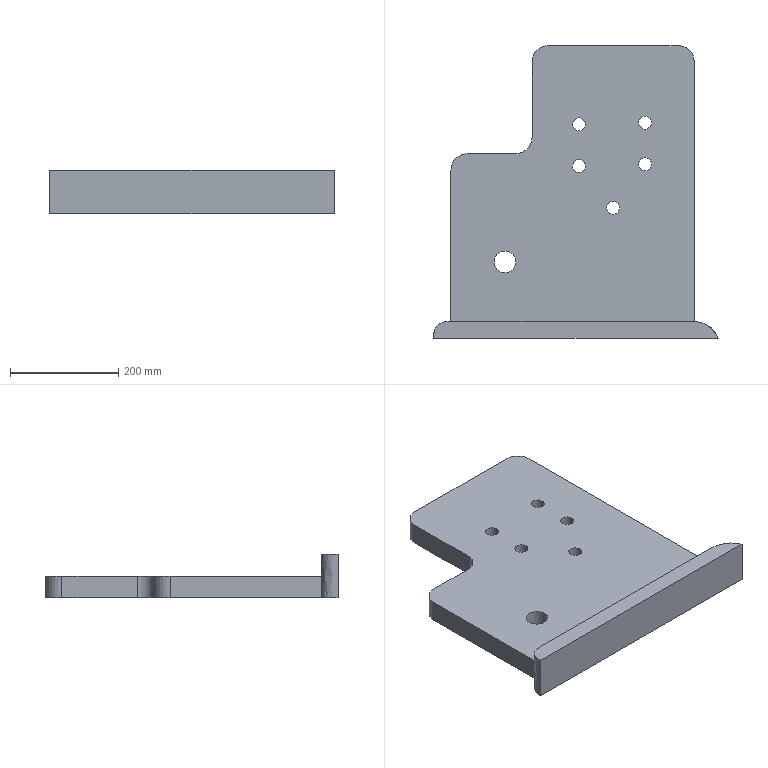Part | SolidWorks | features ICE 8, Extrusion 1, Fillet 1 | 1 solid | 28 faces | box 526.791 x 541.265 x 80 mm | volume 9097852 mm3 | cylinder 16 | plane 10 | spline 2 | commonest cylinder face diameters 24 x10 60 x4 40 x2
STEP:
#1=CARTESIAN_POINT('',(-75.335,154.386,0.));
#2=VERTEX_POINT('',#1);
#3=CARTESIAN_POINT('',(-51.335,154.386,0.));
#4=VERTEX_POINT('',#3);
#5=CARTESIAN_POINT('',(-63.335,154.386,0.));
#6=DIRECTION('',(0.,0.,1.));
#7=DIRECTION('',(1.,0.,0.));
#8=AXIS2_PLACEMENT_3D('',#5,#6,#7);
#9=CIRCLE('',#8,12.);
#10=EDGE_CURVE('',#2,#4,#9,.T.);
#11=ORIENTED_EDGE('',*,*,#10,.F.);
#12=CARTESIAN_POINT('',(-75.335,154.386,40.));
#13=VERTEX_POINT('',#12);
#14=CARTESIAN_POINT('',(-75.335,154.386,-10.));
#15=DIRECTION('',(0.,0.,1.));
#16=VECTOR('',#15,1000.);
#17=LINE('',#14,#16);
#18=EDGE_CURVE('',#2,#13,#17,.T.);
#19=ORIENTED_EDGE('',*,*,#18,.T.);
#20=CARTESIAN_POINT('',(-51.335,154.386,40.));
#21=VERTEX_POINT('',#20);
#22=CARTESIAN_POINT('',(-63.335,154.386,40.));
#23=DIRECTION('',(0.,0.,1.));
#24=DIRECTION('',(1.,0.,0.));
#25=AXIS2_PLACEMENT_3D('',#22,#23,#24);
#26=CIRCLE('',#25,12.);
#27=EDGE_CURVE('',#13,#21,#26,.T.);
#28=ORIENTED_EDGE('',*,*,#27,.T.);
#29=CARTESIAN_POINT('',(-51.335,154.386,-10.));
#30=DIRECTION('',(0.,0.,1.));
#31=VECTOR('',#30,1000.);
#32=LINE('',#29,#31);
#33=EDGE_CURVE('',#4,#21,#32,.T.);
#34=ORIENTED_EDGE('',*,*,#33,.F.);
#35=EDGE_LOOP('',(#11,#19,#28,#34));
#36=FACE_OUTER_BOUND('',#35,.T.);
#37=CARTESIAN_POINT('',(-63.335,154.386,-10.));
#38=DIRECTION('',(0.,0.,1.));
#39=DIRECTION('',(1.,0.,0.));
#40=AXIS2_PLACEMENT_3D('',#37,#38,#39);
#41=CYLINDRICAL_SURFACE('',#40,12.);
#42=ADVANCED_FACE('',(#36),#41,.F.);
#43=CARTESIAN_POINT('',(47.168,157.617,0.));
#44=VERTEX_POINT('',#43);
#45=CARTESIAN_POINT('',(71.168,157.617,0.));
#46=VERTEX_POINT('',#45);
#47=CARTESIAN_POINT('',(59.168,157.617,0.));
#48=DIRECTION('',(0.,0.,1.));
#49=DIRECTION('',(1.,0.,0.));
#50=AXIS2_PLACEMENT_3D('',#47,#48,#49);
#51=CIRCLE('',#50,12.);
#52=EDGE_CURVE('',#44,#46,#51,.T.);
#53=ORIENTED_EDGE('',*,*,#52,.F.);
#54=CARTESIAN_POINT('',(47.168,157.617,40.));
#55=VERTEX_POINT('',#54);
#56=CARTESIAN_POINT('',(47.168,157.617,-10.));
#57=DIRECTION('',(0.,0.,1.));
#58=VECTOR('',#57,1000.);
#59=LINE('',#56,#58);
#60=EDGE_CURVE('',#44,#55,#59,.T.);
#61=ORIENTED_EDGE('',*,*,#60,.T.);
#62=CARTESIAN_POINT('',(71.168,157.617,40.));
#63=VERTEX_POINT('',#62);
#64=CARTESIAN_POINT('',(59.168,157.617,40.));
#65=DIRECTION('',(0.,0.,1.));
#66=DIRECTION('',(1.,0.,0.));
#67=AXIS2_PLACEMENT_3D('',#64,#65,#66);
#68=CIRCLE('',#67,12.);
#69=EDGE_CURVE('',#55,#63,#68,.T.);
#70=ORIENTED_EDGE('',*,*,#69,.T.);
#71=CARTESIAN_POINT('',(71.168,157.617,-10.));
#72=DIRECTION('',(0.,0.,1.));
#73=VECTOR('',#72,1000.);
#74=LINE('',#71,#73);
#75=EDGE_CURVE('',#46,#63,#74,.T.);
#76=ORIENTED_EDGE('',*,*,#75,.F.);
#77=EDGE_LOOP('',(#53,#61,#70,#76));
#78=FACE_OUTER_BOUND('',#77,.T.);
#79=CARTESIAN_POINT('',(59.168,157.617,-10.));
#80=DIRECTION('',(0.,0.,1.));
#81=DIRECTION('',(1.,0.,0.));
#82=AXIS2_PLACEMENT_3D('',#79,#80,#81);
#83=CYLINDRICAL_SURFACE('',#82,12.);
#84=ADVANCED_FACE('',(#78),#83,.F.);
#85=CARTESIAN_POINT('',(-75.335,77.386,0.));
#86=VERTEX_POINT('',#85);
#87=CARTESIAN_POINT('',(-51.335,77.386,0.));
#88=VERTEX_POINT('',#87);
#89=CARTESIAN_POINT('',(-63.335,77.386,0.));
#90=DIRECTION('',(0.,0.,1.));
#91=DIRECTION('',(1.,0.,0.));
#92=AXIS2_PLACEMENT_3D('',#89,#90,#91);
#93=CIRCLE('',#92,12.);
#94=EDGE_CURVE('',#86,#88,#93,.T.);
#95=ORIENTED_EDGE('',*,*,#94,.F.);
#96=CARTESIAN_POINT('',(-75.335,77.386,40.));
#97=VERTEX_POINT('',#96);
#98=CARTESIAN_POINT('',(-75.335,77.386,-50.));
#99=DIRECTION('',(0.,0.,1.));
#100=VECTOR('',#99,1000.);
#101=LINE('',#98,#100);
#102=EDGE_CURVE('',#86,#97,#101,.T.);
#103=ORIENTED_EDGE('',*,*,#102,.T.);
#104=CARTESIAN_POINT('',(-51.335,77.386,40.));
#105=VERTEX_POINT('',#104);
#106=CARTESIAN_POINT('',(-63.335,77.386,40.));
#107=DIRECTION('',(0.,0.,1.));
#108=DIRECTION('',(1.,0.,0.));
#109=AXIS2_PLACEMENT_3D('',#106,#107,#108);
#110=CIRCLE('',#109,12.);
#111=EDGE_CURVE('',#97,#105,#110,.T.);
#112=ORIENTED_EDGE('',*,*,#111,.T.);
#113=CARTESIAN_POINT('',(-51.335,77.386,-50.));
#114=DIRECTION('',(0.,0.,1.));
#115=VECTOR('',#114,1000.);
#116=LINE('',#113,#115);
#117=EDGE_CURVE('',#88,#105,#116,.T.);
#118=ORIENTED_EDGE('',*,*,#117,.F.);
#119=EDGE_LOOP('',(#95,#103,#112,#118));
#120=FACE_OUTER_BOUND('',#119,.T.);
#121=CARTESIAN_POINT('',(-63.335,77.386,-50.));
#122=DIRECTION('',(0.,0.,1.));
#123=DIRECTION('',(1.,0.,0.));
#124=AXIS2_PLACEMENT_3D('',#121,#122,#123);
#125=CYLINDRICAL_SURFACE('',#124,12.);
#126=ADVANCED_FACE('',(#120),#125,.F.);
#127=CARTESIAN_POINT('',(47.168,80.617,0.));
#128=VERTEX_POINT('',#127);
#129=CARTESIAN_POINT('',(71.168,80.617,0.));
#130=VERTEX_POINT('',#129);
#131=CARTESIAN_POINT('',(59.168,80.617,0.));
#132=DIRECTION('',(0.,0.,1.));
#133=DIRECTION('',(1.,0.,0.));
#134=AXIS2_PLACEMENT_3D('',#131,#132,#133);
#135=CIRCLE('',#134,12.);
#136=EDGE_CURVE('',#128,#130,#135,.T.);
#137=ORIENTED_EDGE('',*,*,#136,.F.);
#138=CARTESIAN_POINT('',(47.168,80.617,40.));
#139=VERTEX_POINT('',#138);
#140=CARTESIAN_POINT('',(47.168,80.617,-50.));
#141=DIRECTION('',(0.,0.,1.));
#142=VECTOR('',#141,1000.);
#143=LINE('',#140,#142);
#144=EDGE_CURVE('',#128,#139,#143,.T.);
#145=ORIENTED_EDGE('',*,*,#144,.T.);
#146=CARTESIAN_POINT('',(71.168,80.617,40.));
#147=VERTEX_POINT('',#146);
#148=CARTESIAN_POINT('',(59.168,80.617,40.));
#149=DIRECTION('',(0.,0.,1.));
#150=DIRECTION('',(1.,0.,0.));
#151=AXIS2_PLACEMENT_3D('',#148,#149,#150);
#152=CIRCLE('',#151,12.);
#153=EDGE_CURVE('',#139,#147,#152,.T.);
#154=ORIENTED_EDGE('',*,*,#153,.T.);
#155=CARTESIAN_POINT('',(71.168,80.617,-50.));
#156=DIRECTION('',(0.,0.,1.));
#157=VECTOR('',#156,1000.);
#158=LINE('',#155,#157);
#159=EDGE_CURVE('',#130,#147,#158,.T.);
#160=ORIENTED_EDGE('',*,*,#159,.F.);
#161=EDGE_LOOP('',(#137,#145,#154,#160));
#162=FACE_OUTER_BOUND('',#161,.T.);
#163=CARTESIAN_POINT('',(59.168,80.617,-50.));
#164=DIRECTION('',(0.,0.,1.));
#165=DIRECTION('',(1.,0.,0.));
#166=AXIS2_PLACEMENT_3D('',#163,#164,#165);
#167=CYLINDRICAL_SURFACE('',#166,12.);
#168=ADVANCED_FACE('',(#162),#167,.F.);
#169=CARTESIAN_POINT('',(-12.,0.,0.));
#170=VERTEX_POINT('',#169);
#171=CARTESIAN_POINT('',(12.,0.,0.));
#172=VERTEX_POINT('',#171);
#173=CARTESIAN_POINT('',(0.,0.,0.));
#174=DIRECTION('',(0.,0.,1.));
#175=DIRECTION('',(1.,0.,0.));
#176=AXIS2_PLACEMENT_3D('',#173,#174,#175);
#177=CIRCLE('',#176,12.);
#178=EDGE_CURVE('',#170,#172,#177,.T.);
#179=ORIENTED_EDGE('',*,*,#178,.F.);
#180=CARTESIAN_POINT('',(-12.,0.,40.));
#181=VERTEX_POINT('',#180);
#182=CARTESIAN_POINT('',(-12.,0.,-20.));
#183=DIRECTION('',(0.,0.,1.));
#184=VECTOR('',#183,1000.);
#185=LINE('',#182,#184);
#186=EDGE_CURVE('',#170,#181,#185,.T.);
#187=ORIENTED_EDGE('',*,*,#186,.T.);
#188=CARTESIAN_POINT('',(12.,0.,40.));
#189=VERTEX_POINT('',#188);
#190=CARTESIAN_POINT('',(0.,0.,40.));
#191=DIRECTION('',(0.,0.,1.));
#192=DIRECTION('',(1.,0.,0.));
#193=AXIS2_PLACEMENT_3D('',#190,#191,#192);
#194=CIRCLE('',#193,12.);
#195=EDGE_CURVE('',#181,#189,#194,.T.);
#196=ORIENTED_EDGE('',*,*,#195,.T.);
#197=CARTESIAN_POINT('',(12.,0.,-20.));
#198=DIRECTION('',(0.,0.,1.));
#199=VECTOR('',#198,1000.);
#200=LINE('',#197,#199);
#201=EDGE_CURVE('',#172,#189,#200,.T.);
#202=ORIENTED_EDGE('',*,*,#201,.F.);
#203=EDGE_LOOP('',(#179,#187,#196,#202));
#204=FACE_OUTER_BOUND('',#203,.T.);
#205=CARTESIAN_POINT('',(0.,0.,-20.));
#206=DIRECTION('',(0.,0.,1.));
#207=DIRECTION('',(1.,0.,0.));
#208=AXIS2_PLACEMENT_3D('',#205,#206,#207);
#209=CYLINDRICAL_SURFACE('',#208,12.);
#210=ADVANCED_FACE('',(#204),#209,.F.);
#211=CARTESIAN_POINT('',(-220.,-100.,0.));
#212=VERTEX_POINT('',#211);
#213=CARTESIAN_POINT('',(-180.,-100.,0.));
#214=VERTEX_POINT('',#213);
#215=CARTESIAN_POINT('',(-200.,-100.,0.));
#216=DIRECTION('',(0.,0.,1.));
#217=DIRECTION('',(1.,0.,0.));
#218=AXIS2_PLACEMENT_3D('',#215,#216,#217);
#219=CIRCLE('',#218,20.);
#220=EDGE_CURVE('',#212,#214,#219,.T.);
#221=ORIENTED_EDGE('',*,*,#220,.F.);
#222=CARTESIAN_POINT('',(-220.,-100.,40.));
#223=VERTEX_POINT('',#222);
#224=CARTESIAN_POINT('',(-220.,-100.,0.));
#225=DIRECTION('',(0.,0.,1.));
#226=VECTOR('',#225,1000.);
#227=LINE('',#224,#226);
#228=EDGE_CURVE('',#212,#223,#227,.T.);
#229=ORIENTED_EDGE('',*,*,#228,.T.);
#230=CARTESIAN_POINT('',(-180.,-100.,40.));
#231=VERTEX_POINT('',#230);
#232=CARTESIAN_POINT('',(-200.,-100.,40.));
#233=DIRECTION('',(0.,0.,1.));
#234=DIRECTION('',(1.,0.,0.));
#235=AXIS2_PLACEMENT_3D('',#232,#233,#234);
#236=CIRCLE('',#235,20.);
#237=EDGE_CURVE('',#223,#231,#236,.T.);
#238=ORIENTED_EDGE('',*,*,#237,.T.);
#239=CARTESIAN_POINT('',(-180.,-100.,0.));
#240=DIRECTION('',(0.,0.,1.));
#241=VECTOR('',#240,1000.);
#242=LINE('',#239,#241);
#243=EDGE_CURVE('',#214,#231,#242,.T.);
#244=ORIENTED_EDGE('',*,*,#243,.F.);
#245=EDGE_LOOP('',(#221,#229,#238,#244));
#246=FACE_OUTER_BOUND('',#245,.T.);
#247=CARTESIAN_POINT('',(-200.,-100.,0.));
#248=DIRECTION('',(0.,0.,1.));
#249=DIRECTION('',(1.,0.,0.));
#250=AXIS2_PLACEMENT_3D('',#247,#248,#249);
#251=CYLINDRICAL_SURFACE('',#250,20.);
#252=ADVANCED_FACE('',(#246),#251,.F.);
#253=CARTESIAN_POINT('',(120.,300.,40.));
#254=VERTEX_POINT('',#253);
#255=CARTESIAN_POINT('',(-120.,300.,40.));
#256=VERTEX_POINT('',#255);
#257=CARTESIAN_POINT('',(-300.,300.,40.));
#258=DIRECTION('',(-1.,0.,0.));
#259=VECTOR('',#258,1000.);
#260=LINE('',#257,#259);
#261=EDGE_CURVE('',#254,#256,#260,.T.);
#262=ORIENTED_EDGE('',*,*,#261,.F.);
#263=CARTESIAN_POINT('',(120.,300.,0.));
#264=VERTEX_POINT('',#263);
#265=CARTESIAN_POINT('',(120.,300.,40.));
#266=DIRECTION('',(0.,0.,-1.));
#267=VECTOR('',#266,1000.);
#268=LINE('',#265,#267);
#269=EDGE_CURVE('',#254,#264,#268,.T.);
#270=ORIENTED_EDGE('',*,*,#269,.T.);
#271=CARTESIAN_POINT('',(-120.,300.,0.));
#272=VERTEX_POINT('',#271);
#273=CARTESIAN_POINT('',(-300.,300.,0.));
#274=DIRECTION('',(-1.,0.,0.));
#275=VECTOR('',#274,1000.);
#276=LINE('',#273,#275);
#277=EDGE_CURVE('',#264,#272,#276,.T.);
#278=ORIENTED_EDGE('',*,*,#277,.T.);
#279=CARTESIAN_POINT('',(-120.,300.,40.));
#280=DIRECTION('',(0.,0.,1.));
#281=VECTOR('',#280,1000.);
#282=LINE('',#279,#281);
#283=EDGE_CURVE('',#272,#256,#282,.T.);
#284=ORIENTED_EDGE('',*,*,#283,.T.);
#285=EDGE_LOOP('',(#262,#270,#278,#284));
#286=FACE_OUTER_BOUND('',#285,.T.);
#287=CARTESIAN_POINT('',(-300.,300.,40.));
#288=DIRECTION('',(0.,-1.,0.));
#289=DIRECTION('',(0.,0.,-1.));
#290=AXIS2_PLACEMENT_3D('',#287,#288,#289);
#291=PLANE('',#290);
#292=ADVANCED_FACE('',(#286),#291,.F.);
#293=CARTESIAN_POINT('',(-300.,70.,40.));
#294=VERTEX_POINT('',#293);
#295=CARTESIAN_POINT('',(-300.,-210.,40.));
#296=VERTEX_POINT('',#295);
#297=CARTESIAN_POINT('',(-300.,300.,40.));
#298=DIRECTION('',(0.,-1.,0.));
#299=VECTOR('',#298,1000.);
#300=LINE('',#297,#299);
#301=EDGE_CURVE('',#294,#296,#300,.T.);
#302=ORIENTED_EDGE('',*,*,#301,.F.);
#303=CARTESIAN_POINT('',(-300.,70.,0.));
#304=VERTEX_POINT('',#303);
#305=CARTESIAN_POINT('',(-300.,70.,40.));
#306=DIRECTION('',(0.,0.,-1.));
#307=VECTOR('',#306,1000.);
#308=LINE('',#305,#307);
#309=EDGE_CURVE('',#294,#304,#308,.T.);
#310=ORIENTED_EDGE('',*,*,#309,.T.);
#311=CARTESIAN_POINT('',(-300.,-210.,0.));
#312=VERTEX_POINT('',#311);
#313=CARTESIAN_POINT('',(-300.,300.,0.));
#314=DIRECTION('',(0.,-1.,0.));
#315=VECTOR('',#314,1000.);
#316=LINE('',#313,#315);
#317=EDGE_CURVE('',#304,#312,#316,.T.);
#318=ORIENTED_EDGE('',*,*,#317,.T.);
#319=CARTESIAN_POINT('',(-300.,-210.,-60.));
#320=DIRECTION('',(0.,0.,1.));
#321=VECTOR('',#320,1000.);
#322=LINE('',#319,#321);
#323=EDGE_CURVE('',#312,#296,#322,.T.);
#324=ORIENTED_EDGE('',*,*,#323,.T.);
#325=EDGE_LOOP('',(#302,#310,#318,#324));
#326=FACE_OUTER_BOUND('',#325,.T.);
#327=CARTESIAN_POINT('',(-300.,300.,40.));
#328=DIRECTION('',(1.,0.,0.));
#329=DIRECTION('',(0.,1.,0.));
#330=AXIS2_PLACEMENT_3D('',#327,#328,#329);
#331=PLANE('',#330);
#332=ADVANCED_FACE('',(#326),#331,.F.);
#333=CARTESIAN_POINT('',(-63.335,154.386,40.));
#334=DIRECTION('',(0.,0.,1.));
#335=DIRECTION('',(1.,0.,0.));
#336=AXIS2_PLACEMENT_3D('',#333,#334,#335);
#337=CIRCLE('',#336,12.);
#338=EDGE_CURVE('',#21,#13,#337,.T.);
#339=ORIENTED_EDGE('',*,*,#338,.F.);
#340=ORIENTED_EDGE('',*,*,#27,.F.);
#341=EDGE_LOOP('',(#339,#340));
#342=FACE_BOUND('',#341,.T.);
#343=CARTESIAN_POINT('',(59.168,157.617,40.));
#344=DIRECTION('',(0.,0.,1.));
#345=DIRECTION('',(1.,0.,0.));
#346=AXIS2_PLACEMENT_3D('',#343,#344,#345);
#347=CIRCLE('',#346,12.);
#348=EDGE_CURVE('',#63,#55,#347,.T.);
#349=ORIENTED_EDGE('',*,*,#348,.F.);
#350=ORIENTED_EDGE('',*,*,#69,.F.);
#351=EDGE_LOOP('',(#349,#350));
#352=FACE_BOUND('',#351,.T.);
#353=CARTESIAN_POINT('',(-270.,100.,40.));
#354=VERTEX_POINT('',#353);
#355=CARTESIAN_POINT('',(-180.,100.,40.));
#356=VERTEX_POINT('',#355);
#357=CARTESIAN_POINT('',(-300.,100.,40.));
#358=DIRECTION('',(1.,0.,0.));
#359=VECTOR('',#358,1000.);
#360=LINE('',#357,#359);
#361=EDGE_CURVE('',#354,#356,#360,.T.);
#362=ORIENTED_EDGE('',*,*,#361,.F.);
#363=CARTESIAN_POINT('',(-270.,70.,40.));
#364=DIRECTION('',(0.,0.,1.));
#365=DIRECTION('',(1.,0.,0.));
#366=AXIS2_PLACEMENT_3D('',#363,#364,#365);
#367=CIRCLE('',#366,30.);
#368=EDGE_CURVE('',#354,#294,#367,.T.);
#369=ORIENTED_EDGE('',*,*,#368,.T.);
#370=ORIENTED_EDGE('',*,*,#301,.T.);
#371=CARTESIAN_POINT('',(150.,-210.,40.));
#372=VERTEX_POINT('',#371);
#373=CARTESIAN_POINT('',(-300.,-210.,40.));
#374=DIRECTION('',(-1.,0.,0.));
#375=VECTOR('',#374,1000.);
#376=LINE('',#373,#375);
#377=EDGE_CURVE('',#372,#296,#376,.T.);
#378=ORIENTED_EDGE('',*,*,#377,.F.);
#379=CARTESIAN_POINT('',(150.,270.,40.));
#380=VERTEX_POINT('',#379);
#381=CARTESIAN_POINT('',(150.,300.,40.));
#382=DIRECTION('',(0.,-1.,0.));
#383=VECTOR('',#382,1000.);
#384=LINE('',#381,#383);
#385=EDGE_CURVE('',#380,#372,#384,.T.);
#386=ORIENTED_EDGE('',*,*,#385,.F.);
#387=CARTESIAN_POINT('',(120.,270.,40.));
#388=DIRECTION('',(0.,0.,1.));
#389=DIRECTION('',(1.,0.,0.));
#390=AXIS2_PLACEMENT_3D('',#387,#388,#389);
#391=CIRCLE('',#390,30.);
#392=EDGE_CURVE('',#380,#254,#391,.T.);
#393=ORIENTED_EDGE('',*,*,#392,.T.);
#394=ORIENTED_EDGE('',*,*,#261,.T.);
#395=CARTESIAN_POINT('',(-150.,270.,40.));
#396=VERTEX_POINT('',#395);
#397=CARTESIAN_POINT('',(-120.,270.,40.));
#398=DIRECTION('',(0.,0.,1.));
#399=DIRECTION('',(1.,0.,0.));
#400=AXIS2_PLACEMENT_3D('',#397,#398,#399);
#401=CIRCLE('',#400,30.);
#402=EDGE_CURVE('',#256,#396,#401,.T.);
#403=ORIENTED_EDGE('',*,*,#402,.T.);
#404=CARTESIAN_POINT('',(-150.,130.,40.));
#405=VERTEX_POINT('',#404);
#406=CARTESIAN_POINT('',(-150.,300.,40.));
#407=DIRECTION('',(0.,1.,0.));
#408=VECTOR('',#407,1000.);
#409=LINE('',#406,#408);
#410=EDGE_CURVE('',#405,#396,#409,.T.);
#411=ORIENTED_EDGE('',*,*,#410,.F.);
#412=CARTESIAN_POINT('',(-180.,130.,40.));
#413=DIRECTION('',(0.,0.,-1.));
#414=DIRECTION('',(1.,0.,0.));
#415=AXIS2_PLACEMENT_3D('',#412,#413,#414);
#416=CIRCLE('',#415,30.);
#417=EDGE_CURVE('',#405,#356,#416,.T.);
#418=ORIENTED_EDGE('',*,*,#417,.T.);
#419=EDGE_LOOP('',(#362,#369,#370,#378,#386,#393,#394,#403,#411,#418));
#420=FACE_OUTER_BOUND('',#419,.T.);
#421=CARTESIAN_POINT('',(-63.335,77.386,40.));
#422=DIRECTION('',(0.,0.,1.));
#423=DIRECTION('',(1.,0.,0.));
#424=AXIS2_PLACEMENT_3D('',#421,#422,#423);
#425=CIRCLE('',#424,12.);
#426=EDGE_CURVE('',#105,#97,#425,.T.);
#427=ORIENTED_EDGE('',*,*,#426,.F.);
#428=ORIENTED_EDGE('',*,*,#111,.F.);
#429=EDGE_LOOP('',(#427,#428));
#430=FACE_BOUND('',#429,.T.);
#431=CARTESIAN_POINT('',(59.168,80.617,40.));
#432=DIRECTION('',(0.,0.,1.));
#433=DIRECTION('',(1.,0.,0.));
#434=AXIS2_PLACEMENT_3D('',#431,#432,#433);
#435=CIRCLE('',#434,12.);
#436=EDGE_CURVE('',#147,#139,#435,.T.);
#437=ORIENTED_EDGE('',*,*,#436,.F.);
#438=ORIENTED_EDGE('',*,*,#153,.F.);
#439=EDGE_LOOP('',(#437,#438));
#440=FACE_BOUND('',#439,.T.);
#441=CARTESIAN_POINT('',(0.,0.,40.));
#442=DIRECTION('',(0.,0.,1.));
#443=DIRECTION('',(1.,0.,0.));
#444=AXIS2_PLACEMENT_3D('',#441,#442,#443);
#445=CIRCLE('',#444,12.);
#446=EDGE_CURVE('',#189,#181,#445,.T.);
#447=ORIENTED_EDGE('',*,*,#446,.F.);
#448=ORIENTED_EDGE('',*,*,#195,.F.);
#449=EDGE_LOOP('',(#447,#448));
#450=FACE_BOUND('',#449,.T.);
#451=CARTESIAN_POINT('',(-200.,-100.,40.));
#452=DIRECTION('',(0.,0.,1.));
#453=DIRECTION('',(1.,0.,0.));
#454=AXIS2_PLACEMENT_3D('',#451,#452,#453);
#455=CIRCLE('',#454,20.);
#456=EDGE_CURVE('',#231,#223,#455,.T.);
#457=ORIENTED_EDGE('',*,*,#456,.F.);
#458=ORIENTED_EDGE('',*,*,#237,.F.);
#459=EDGE_LOOP('',(#457,#458));
#460=FACE_BOUND('',#459,.T.);
#461=CARTESIAN_POINT('',(0.,0.,40.));
#462=DIRECTION('',(0.,0.,1.));
#463=DIRECTION('',(1.,0.,0.));
#464=AXIS2_PLACEMENT_3D('',#461,#462,#463);
#465=PLANE('',#464);
#466=ADVANCED_FACE('',(#342,#352,#420,#430,#440,#450,#460),#465,.T.);
#467=CARTESIAN_POINT('',(-63.335,154.386,0.));
#468=DIRECTION('',(0.,0.,1.));
#469=DIRECTION('',(1.,0.,0.));
#470=AXIS2_PLACEMENT_3D('',#467,#468,#469);
#471=CIRCLE('',#470,12.);
#472=EDGE_CURVE('',#4,#2,#471,.T.);
#473=ORIENTED_EDGE('',*,*,#472,.T.);
#474=ORIENTED_EDGE('',*,*,#10,.T.);
#475=EDGE_LOOP('',(#473,#474));
#476=FACE_BOUND('',#475,.T.);
#477=CARTESIAN_POINT('',(59.168,157.617,0.));
#478=DIRECTION('',(0.,0.,1.));
#479=DIRECTION('',(1.,0.,0.));
#480=AXIS2_PLACEMENT_3D('',#477,#478,#479);
#481=CIRCLE('',#480,12.);
#482=EDGE_CURVE('',#46,#44,#481,.T.);
#483=ORIENTED_EDGE('',*,*,#482,.T.);
#484=ORIENTED_EDGE('',*,*,#52,.T.);
#485=EDGE_LOOP('',(#483,#484));
#486=FACE_BOUND('',#485,.T.);
#487=CARTESIAN_POINT('',(-63.335,77.386,0.));
#488=DIRECTION('',(0.,0.,1.));
#489=DIRECTION('',(1.,0.,0.));
#490=AXIS2_PLACEMENT_3D('',#487,#488,#489);
#491=CIRCLE('',#490,12.);
#492=EDGE_CURVE('',#88,#86,#491,.T.);
#493=ORIENTED_EDGE('',*,*,#492,.T.);
#494=ORIENTED_EDGE('',*,*,#94,.T.);
#495=EDGE_LOOP('',(#493,#494));
#496=FACE_BOUND('',#495,.T.);
#497=CARTESIAN_POINT('',(59.168,80.617,0.));
#498=DIRECTION('',(0.,0.,1.));
#499=DIRECTION('',(1.,0.,0.));
#500=AXIS2_PLACEMENT_3D('',#497,#498,#499);
#501=CIRCLE('',#500,12.);
#502=EDGE_CURVE('',#130,#128,#501,.T.);
#503=ORIENTED_EDGE('',*,*,#502,.T.);
#504=ORIENTED_EDGE('',*,*,#136,.T.);
#505=EDGE_LOOP('',(#503,#504));
#506=FACE_BOUND('',#505,.T.);
#507=CARTESIAN_POINT('',(0.,0.,0.));
#508=DIRECTION('',(0.,0.,1.));
#509=DIRECTION('',(1.,0.,0.));
#510=AXIS2_PLACEMENT_3D('',#507,#508,#509);
#511=CIRCLE('',#510,12.);
#512=EDGE_CURVE('',#172,#170,#511,.T.);
#513=ORIENTED_EDGE('',*,*,#512,.T.);
#514=ORIENTED_EDGE('',*,*,#178,.T.);
#515=EDGE_LOOP('',(#513,#514));
#516=FACE_BOUND('',#515,.T.);
#517=CARTESIAN_POINT('',(-200.,-100.,0.));
#518=DIRECTION('',(0.,0.,1.));
#519=DIRECTION('',(1.,0.,0.));
#520=AXIS2_PLACEMENT_3D('',#517,#518,#519);
#521=CIRCLE('',#520,20.);
#522=EDGE_CURVE('',#214,#212,#521,.T.);
#523=ORIENTED_EDGE('',*,*,#522,.T.);
#524=ORIENTED_EDGE('',*,*,#220,.T.);
#525=EDGE_LOOP('',(#523,#524));
#526=FACE_BOUND('',#525,.T.);
#527=ORIENTED_EDGE('',*,*,#317,.F.);
#528=CARTESIAN_POINT('',(-270.,100.,0.));
#529=VERTEX_POINT('',#528);
#530=CARTESIAN_POINT('',(-270.,70.,0.));
#531=DIRECTION('',(0.,0.,-1.));
#532=DIRECTION('',(1.,0.,0.));
#533=AXIS2_PLACEMENT_3D('',#530,#531,#532);
#534=CIRCLE('',#533,30.);
#535=EDGE_CURVE('',#304,#529,#534,.T.);
#536=ORIENTED_EDGE('',*,*,#535,.T.);
#537=CARTESIAN_POINT('',(-180.,100.,0.));
#538=VERTEX_POINT('',#537);
#539=CARTESIAN_POINT('',(0.,100.,0.));
#540=DIRECTION('',(1.,0.,0.));
#541=VECTOR('',#540,1000.);
#542=LINE('',#539,#541);
#543=EDGE_CURVE('',#529,#538,#542,.T.);
#544=ORIENTED_EDGE('',*,*,#543,.T.);
#545=CARTESIAN_POINT('',(-150.,130.,0.));
#546=VERTEX_POINT('',#545);
#547=CARTESIAN_POINT('',(-180.,130.,0.));
#548=DIRECTION('',(0.,0.,1.));
#549=DIRECTION('',(1.,0.,0.));
#550=AXIS2_PLACEMENT_3D('',#547,#548,#549);
#551=CIRCLE('',#550,30.);
#552=EDGE_CURVE('',#538,#546,#551,.T.);
#553=ORIENTED_EDGE('',*,*,#552,.T.);
#554=CARTESIAN_POINT('',(-150.,270.,0.));
#555=VERTEX_POINT('',#554);
#556=CARTESIAN_POINT('',(-150.,0.,0.));
#557=DIRECTION('',(0.,1.,0.));
#558=VECTOR('',#557,1000.);
#559=LINE('',#556,#558);
#560=EDGE_CURVE('',#546,#555,#559,.T.);
#561=ORIENTED_EDGE('',*,*,#560,.T.);
#562=CARTESIAN_POINT('',(-120.,270.,0.));
#563=DIRECTION('',(0.,0.,-1.));
#564=DIRECTION('',(1.,0.,0.));
#565=AXIS2_PLACEMENT_3D('',#562,#563,#564);
#566=CIRCLE('',#565,30.);
#567=EDGE_CURVE('',#555,#272,#566,.T.);
#568=ORIENTED_EDGE('',*,*,#567,.T.);
#569=ORIENTED_EDGE('',*,*,#277,.F.);
#570=CARTESIAN_POINT('',(150.,270.,0.));
#571=VERTEX_POINT('',#570);
#572=CARTESIAN_POINT('',(120.,270.,0.));
#573=DIRECTION('',(0.,0.,-1.));
#574=DIRECTION('',(1.,0.,0.));
#575=AXIS2_PLACEMENT_3D('',#572,#573,#574);
#576=CIRCLE('',#575,30.);
#577=EDGE_CURVE('',#264,#571,#576,.T.);
#578=ORIENTED_EDGE('',*,*,#577,.T.);
#579=CARTESIAN_POINT('',(150.,-210.,0.));
#580=VERTEX_POINT('',#579);
#581=CARTESIAN_POINT('',(150.,0.,0.));
#582=DIRECTION('',(0.,-1.,0.));
#583=VECTOR('',#582,1000.);
#584=LINE('',#581,#583);
#585=EDGE_CURVE('',#571,#580,#584,.T.);
#586=ORIENTED_EDGE('',*,*,#585,.T.);
#587=CARTESIAN_POINT('',(194.702,-241.265,0.));
#588=VERTEX_POINT('',#587);
#589=CARTESIAN_POINT('',(150.,-210.,0.));
#590=CARTESIAN_POINT('',(181.313,-212.059,0.));
#591=CARTESIAN_POINT('',(194.702,-241.265,0.));
#592=B_SPLINE_CURVE_WITH_KNOTS('',2,(#589,#590,#591),.UNSPECIFIED.,.F.,.F.,(3,3),(0.,1.),.UNSPECIFIED.);
#593=EDGE_CURVE('',#580,#588,#592,.T.);
#594=ORIENTED_EDGE('',*,*,#593,.T.);
#595=CARTESIAN_POINT('',(-332.054,-241.265,0.));
#596=VERTEX_POINT('',#595);
#597=CARTESIAN_POINT('',(194.702,-241.265,0.));
#598=DIRECTION('',(-1.,0.,0.));
#599=VECTOR('',#598,1000.);
#600=LINE('',#597,#599);
#601=EDGE_CURVE('',#588,#596,#600,.T.);
#602=ORIENTED_EDGE('',*,*,#601,.T.);
#603=CARTESIAN_POINT('',(-332.054,-241.265,0.));
#604=CARTESIAN_POINT('',(-333.146,-208.556,0.));
#605=CARTESIAN_POINT('',(-300.,-210.,0.));
#606=B_SPLINE_CURVE_WITH_KNOTS('',2,(#603,#604,#605),.UNSPECIFIED.,.F.,.F.,(3,3),(0.,1.),.UNSPECIFIED.);
#607=EDGE_CURVE('',#596,#312,#606,.T.);
#608=ORIENTED_EDGE('',*,*,#607,.T.);
#609=EDGE_LOOP('',(#527,#536,#544,#553,#561,#568,#569,#578,#586,#594,#602,#608));
#610=FACE_OUTER_BOUND('',#609,.T.);
#611=CARTESIAN_POINT('',(0.,0.,0.));
#612=DIRECTION('',(0.,0.,1.));
#613=DIRECTION('',(1.,0.,0.));
#614=AXIS2_PLACEMENT_3D('',#611,#612,#613);
#615=PLANE('',#614);
#616=ADVANCED_FACE('',(#476,#486,#496,#506,#516,#526,#610),#615,.F.);
#617=ORIENTED_EDGE('',*,*,#228,.F.);
#618=ORIENTED_EDGE('',*,*,#522,.F.);
#619=ORIENTED_EDGE('',*,*,#243,.T.);
#620=ORIENTED_EDGE('',*,*,#456,.T.);
#621=EDGE_LOOP('',(#617,#618,#619,#620));
#622=FACE_OUTER_BOUND('',#621,.T.);
#623=CARTESIAN_POINT('',(-200.,-100.,0.));
#624=DIRECTION('',(0.,0.,1.));
#625=DIRECTION('',(1.,0.,0.));
#626=AXIS2_PLACEMENT_3D('',#623,#624,#625);
#627=CYLINDRICAL_SURFACE('',#626,20.);
#628=ADVANCED_FACE('',(#622),#627,.F.);
#629=ORIENTED_EDGE('',*,*,#186,.F.);
#630=ORIENTED_EDGE('',*,*,#512,.F.);
#631=ORIENTED_EDGE('',*,*,#201,.T.);
#632=ORIENTED_EDGE('',*,*,#446,.T.);
#633=EDGE_LOOP('',(#629,#630,#631,#632));
#634=FACE_OUTER_BOUND('',#633,.T.);
#635=CARTESIAN_POINT('',(0.,0.,-20.));
#636=DIRECTION('',(0.,0.,1.));
#637=DIRECTION('',(1.,0.,0.));
#638=AXIS2_PLACEMENT_3D('',#635,#636,#637);
#639=CYLINDRICAL_SURFACE('',#638,12.);
#640=ADVANCED_FACE('',(#634),#639,.F.);
#641=ORIENTED_EDGE('',*,*,#144,.F.);
#642=ORIENTED_EDGE('',*,*,#502,.F.);
#643=ORIENTED_EDGE('',*,*,#159,.T.);
#644=ORIENTED_EDGE('',*,*,#436,.T.);
#645=EDGE_LOOP('',(#641,#642,#643,#644));
#646=FACE_OUTER_BOUND('',#645,.T.);
#647=CARTESIAN_POINT('',(59.168,80.617,-50.));
#648=DIRECTION('',(0.,0.,1.));
#649=DIRECTION('',(1.,0.,0.));
#650=AXIS2_PLACEMENT_3D('',#647,#648,#649);
#651=CYLINDRICAL_SURFACE('',#650,12.);
#652=ADVANCED_FACE('',(#646),#651,.F.);
#653=ORIENTED_EDGE('',*,*,#102,.F.);
#654=ORIENTED_EDGE('',*,*,#492,.F.);
#655=ORIENTED_EDGE('',*,*,#117,.T.);
#656=ORIENTED_EDGE('',*,*,#426,.T.);
#657=EDGE_LOOP('',(#653,#654,#655,#656));
#658=FACE_OUTER_BOUND('',#657,.T.);
#659=CARTESIAN_POINT('',(-63.335,77.386,-50.));
#660=DIRECTION('',(0.,0.,1.));
#661=DIRECTION('',(1.,0.,0.));
#662=AXIS2_PLACEMENT_3D('',#659,#660,#661);
#663=CYLINDRICAL_SURFACE('',#662,12.);
#664=ADVANCED_FACE('',(#658),#663,.F.);
#665=ORIENTED_EDGE('',*,*,#585,.F.);
#666=CARTESIAN_POINT('',(150.,270.,-60.));
#667=DIRECTION('',(0.,0.,1.));
#668=VECTOR('',#667,1000.);
#669=LINE('',#666,#668);
#670=EDGE_CURVE('',#571,#380,#669,.T.);
#671=ORIENTED_EDGE('',*,*,#670,.T.);
#672=ORIENTED_EDGE('',*,*,#385,.T.);
#673=CARTESIAN_POINT('',(150.,-210.,-60.));
#674=DIRECTION('',(0.,0.,-1.));
#675=VECTOR('',#674,1000.);
#676=LINE('',#673,#675);
#677=EDGE_CURVE('',#372,#580,#676,.T.);
#678=ORIENTED_EDGE('',*,*,#677,.T.);
#679=EDGE_LOOP('',(#665,#671,#672,#678));
#680=FACE_OUTER_BOUND('',#679,.T.);
#681=CARTESIAN_POINT('',(150.,300.,-60.));
#682=DIRECTION('',(-1.,0.,0.));
#683=DIRECTION('',(0.,-1.,0.));
#684=AXIS2_PLACEMENT_3D('',#681,#682,#683);
#685=PLANE('',#684);
#686=ADVANCED_FACE('',(#680),#685,.F.);
#687=ORIENTED_EDGE('',*,*,#560,.F.);
#688=CARTESIAN_POINT('',(-150.,130.,40.));
#689=DIRECTION('',(0.,0.,1.));
#690=VECTOR('',#689,1000.);
#691=LINE('',#688,#690);
#692=EDGE_CURVE('',#546,#405,#691,.T.);
#693=ORIENTED_EDGE('',*,*,#692,.T.);
#694=ORIENTED_EDGE('',*,*,#410,.T.);
#695=CARTESIAN_POINT('',(-150.,270.,-60.));
#696=DIRECTION('',(0.,0.,-1.));
#697=VECTOR('',#696,1000.);
#698=LINE('',#695,#697);
#699=EDGE_CURVE('',#396,#555,#698,.T.);
#700=ORIENTED_EDGE('',*,*,#699,.T.);
#701=EDGE_LOOP('',(#687,#693,#694,#700));
#702=FACE_OUTER_BOUND('',#701,.T.);
#703=CARTESIAN_POINT('',(-150.,300.,-60.));
#704=DIRECTION('',(1.,0.,0.));
#705=DIRECTION('',(0.,1.,0.));
#706=AXIS2_PLACEMENT_3D('',#703,#704,#705);
#707=PLANE('',#706);
#708=ADVANCED_FACE('',(#702),#707,.F.);
#709=ORIENTED_EDGE('',*,*,#543,.F.);
#710=CARTESIAN_POINT('',(-270.,100.,-60.));
#711=DIRECTION('',(0.,0.,1.));
#712=VECTOR('',#711,1000.);
#713=LINE('',#710,#712);
#714=EDGE_CURVE('',#529,#354,#713,.T.);
#715=ORIENTED_EDGE('',*,*,#714,.T.);
#716=ORIENTED_EDGE('',*,*,#361,.T.);
#717=CARTESIAN_POINT('',(-180.,100.,0.));
#718=DIRECTION('',(0.,0.,-1.));
#719=VECTOR('',#718,1000.);
#720=LINE('',#717,#719);
#721=EDGE_CURVE('',#356,#538,#720,.T.);
#722=ORIENTED_EDGE('',*,*,#721,.T.);
#723=EDGE_LOOP('',(#709,#715,#716,#722));
#724=FACE_OUTER_BOUND('',#723,.T.);
#725=CARTESIAN_POINT('',(-300.,100.,-60.));
#726=DIRECTION('',(0.,-1.,0.));
#727=DIRECTION('',(0.,0.,-1.));
#728=AXIS2_PLACEMENT_3D('',#725,#726,#727);
#729=PLANE('',#728);
#730=ADVANCED_FACE('',(#724),#729,.F.);
#731=ORIENTED_EDGE('',*,*,#60,.F.);
#732=ORIENTED_EDGE('',*,*,#482,.F.);
#733=ORIENTED_EDGE('',*,*,#75,.T.);
#734=ORIENTED_EDGE('',*,*,#348,.T.);
#735=EDGE_LOOP('',(#731,#732,#733,#734));
#736=FACE_OUTER_BOUND('',#735,.T.);
#737=CARTESIAN_POINT('',(59.168,157.617,-10.));
#738=DIRECTION('',(0.,0.,1.));
#739=DIRECTION('',(1.,0.,0.));
#740=AXIS2_PLACEMENT_3D('',#737,#738,#739);
#741=CYLINDRICAL_SURFACE('',#740,12.);
#742=ADVANCED_FACE('',(#736),#741,.F.);
#743=ORIENTED_EDGE('',*,*,#18,.F.);
#744=ORIENTED_EDGE('',*,*,#472,.F.);
#745=ORIENTED_EDGE('',*,*,#33,.T.);
#746=ORIENTED_EDGE('',*,*,#338,.T.);
#747=EDGE_LOOP('',(#743,#744,#745,#746));
#748=FACE_OUTER_BOUND('',#747,.T.);
#749=CARTESIAN_POINT('',(-63.335,154.386,-10.));
#750=DIRECTION('',(0.,0.,1.));
#751=DIRECTION('',(1.,0.,0.));
#752=AXIS2_PLACEMENT_3D('',#749,#750,#751);
#753=CYLINDRICAL_SURFACE('',#752,12.);
#754=ADVANCED_FACE('',(#748),#753,.F.);
#755=ORIENTED_EDGE('',*,*,#535,.F.);
#756=ORIENTED_EDGE('',*,*,#309,.F.);
#757=ORIENTED_EDGE('',*,*,#368,.F.);
#758=ORIENTED_EDGE('',*,*,#714,.F.);
#759=EDGE_LOOP('',(#755,#756,#757,#758));
#760=FACE_OUTER_BOUND('',#759,.T.);
#761=CARTESIAN_POINT('',(-270.,70.,-60.));
#762=DIRECTION('',(0.,0.,1.));
#763=DIRECTION('',(1.,0.,0.));
#764=AXIS2_PLACEMENT_3D('',#761,#762,#763);
#765=CYLINDRICAL_SURFACE('',#764,30.);
#766=ADVANCED_FACE('',(#760),#765,.T.);
#767=ORIENTED_EDGE('',*,*,#552,.F.);
#768=ORIENTED_EDGE('',*,*,#721,.F.);
#769=ORIENTED_EDGE('',*,*,#417,.F.);
#770=ORIENTED_EDGE('',*,*,#692,.F.);
#771=EDGE_LOOP('',(#767,#768,#769,#770));
#772=FACE_OUTER_BOUND('',#771,.T.);
#773=CARTESIAN_POINT('',(-180.,130.,-60.));
#774=DIRECTION('',(0.,0.,-1.));
#775=DIRECTION('',(-1.,0.,0.));
#776=AXIS2_PLACEMENT_3D('',#773,#774,#775);
#777=CYLINDRICAL_SURFACE('',#776,30.);
#778=ADVANCED_FACE('',(#772),#777,.F.);
#779=ORIENTED_EDGE('',*,*,#577,.F.);
#780=ORIENTED_EDGE('',*,*,#269,.F.);
#781=ORIENTED_EDGE('',*,*,#392,.F.);
#782=ORIENTED_EDGE('',*,*,#670,.F.);
#783=EDGE_LOOP('',(#779,#780,#781,#782));
#784=FACE_OUTER_BOUND('',#783,.T.);
#785=CARTESIAN_POINT('',(120.,270.,-60.));
#786=DIRECTION('',(0.,0.,1.));
#787=DIRECTION('',(1.,0.,0.));
#788=AXIS2_PLACEMENT_3D('',#785,#786,#787);
#789=CYLINDRICAL_SURFACE('',#788,30.);
#790=ADVANCED_FACE('',(#784),#789,.T.);
#791=ORIENTED_EDGE('',*,*,#567,.F.);
#792=ORIENTED_EDGE('',*,*,#699,.F.);
#793=ORIENTED_EDGE('',*,*,#402,.F.);
#794=ORIENTED_EDGE('',*,*,#283,.F.);
#795=EDGE_LOOP('',(#791,#792,#793,#794));
#796=FACE_OUTER_BOUND('',#795,.T.);
#797=CARTESIAN_POINT('',(-120.,270.,40.));
#798=DIRECTION('',(0.,0.,1.));
#799=DIRECTION('',(1.,0.,0.));
#800=AXIS2_PLACEMENT_3D('',#797,#798,#799);
#801=CYLINDRICAL_SURFACE('',#800,30.);
#802=ADVANCED_FACE('',(#796),#801,.T.);
#803=ORIENTED_EDGE('',*,*,#593,.F.);
#804=ORIENTED_EDGE('',*,*,#677,.F.);
#805=CARTESIAN_POINT('',(150.,-210.,80.));
#806=VERTEX_POINT('',#805);
#807=CARTESIAN_POINT('',(150.,-210.,80.));
#808=DIRECTION('',(0.,0.,-1.));
#809=VECTOR('',#808,1000.);
#810=LINE('',#807,#809);
#811=EDGE_CURVE('',#806,#372,#810,.T.);
#812=ORIENTED_EDGE('',*,*,#811,.F.);
#813=CARTESIAN_POINT('',(194.702,-241.265,80.));
#814=VERTEX_POINT('',#813);
#815=CARTESIAN_POINT('',(150.,-210.,80.));
#816=CARTESIAN_POINT('',(181.313,-212.059,80.));
#817=CARTESIAN_POINT('',(194.702,-241.265,80.));
#818=B_SPLINE_CURVE_WITH_KNOTS('',2,(#815,#816,#817),.UNSPECIFIED.,.F.,.F.,(3,3),(0.,1.),.UNSPECIFIED.);
#819=EDGE_CURVE('',#806,#814,#818,.T.);
#820=ORIENTED_EDGE('',*,*,#819,.T.);
#821=CARTESIAN_POINT('',(194.702,-241.265,80.));
#822=DIRECTION('',(0.,0.,-1.));
#823=VECTOR('',#822,1000.);
#824=LINE('',#821,#823);
#825=EDGE_CURVE('',#814,#588,#824,.T.);
#826=ORIENTED_EDGE('',*,*,#825,.T.);
#827=EDGE_LOOP('',(#803,#804,#812,#820,#826));
#828=FACE_OUTER_BOUND('',#827,.T.);
#829=CARTESIAN_POINT('',(150.,-210.,80.));
#830=CARTESIAN_POINT('',(150.,-210.,0.));
#831=CARTESIAN_POINT('',(181.313,-212.059,80.));
#832=CARTESIAN_POINT('',(181.313,-212.059,0.));
#833=CARTESIAN_POINT('',(194.702,-241.265,80.));
#834=CARTESIAN_POINT('',(194.702,-241.265,0.));
#835=B_SPLINE_SURFACE_WITH_KNOTS('',2,1,((#829,#830),(#831,#832),(#833,#834)),.UNSPECIFIED.,.F.,.F.,.F.,(3,3),(2,2),(0.,1.),(0.,1.),.UNSPECIFIED.);
#836=ADVANCED_FACE('',(#828),#835,.T.);
#837=ORIENTED_EDGE('',*,*,#811,.T.);
#838=ORIENTED_EDGE('',*,*,#377,.T.);
#839=CARTESIAN_POINT('',(-300.,-210.,80.));
#840=VERTEX_POINT('',#839);
#841=CARTESIAN_POINT('',(-300.,-210.,80.));
#842=DIRECTION('',(0.,0.,-1.));
#843=VECTOR('',#842,1000.);
#844=LINE('',#841,#843);
#845=EDGE_CURVE('',#840,#296,#844,.T.);
#846=ORIENTED_EDGE('',*,*,#845,.F.);
#847=CARTESIAN_POINT('',(150.,-210.,80.));
#848=DIRECTION('',(1.,0.,0.));
#849=VECTOR('',#848,1000.);
#850=LINE('',#847,#849);
#851=EDGE_CURVE('',#840,#806,#850,.T.);
#852=ORIENTED_EDGE('',*,*,#851,.T.);
#853=EDGE_LOOP('',(#837,#838,#846,#852));
#854=FACE_OUTER_BOUND('',#853,.T.);
#855=CARTESIAN_POINT('',(150.,-210.,80.));
#856=DIRECTION('',(0.,1.,0.));
#857=DIRECTION('',(-1.,0.,0.));
#858=AXIS2_PLACEMENT_3D('',#855,#856,#857);
#859=PLANE('',#858);
#860=ADVANCED_FACE('',(#854),#859,.T.);
#861=ORIENTED_EDGE('',*,*,#607,.F.);
#862=CARTESIAN_POINT('',(-332.054,-241.265,80.));
#863=VERTEX_POINT('',#862);
#864=CARTESIAN_POINT('',(-332.054,-241.265,80.));
#865=DIRECTION('',(0.,0.,-1.));
#866=VECTOR('',#865,1000.);
#867=LINE('',#864,#866);
#868=EDGE_CURVE('',#863,#596,#867,.T.);
#869=ORIENTED_EDGE('',*,*,#868,.F.);
#870=CARTESIAN_POINT('',(-332.054,-241.265,80.));
#871=CARTESIAN_POINT('',(-333.146,-208.556,80.));
#872=CARTESIAN_POINT('',(-300.,-210.,80.));
#873=B_SPLINE_CURVE_WITH_KNOTS('',2,(#870,#871,#872),.UNSPECIFIED.,.F.,.F.,(3,3),(0.,1.),.UNSPECIFIED.);
#874=EDGE_CURVE('',#863,#840,#873,.T.);
#875=ORIENTED_EDGE('',*,*,#874,.T.);
#876=ORIENTED_EDGE('',*,*,#845,.T.);
#877=ORIENTED_EDGE('',*,*,#323,.F.);
#878=EDGE_LOOP('',(#861,#869,#875,#876,#877));
#879=FACE_OUTER_BOUND('',#878,.T.);
#880=CARTESIAN_POINT('',(-332.054,-241.265,80.));
#881=CARTESIAN_POINT('',(-332.054,-241.265,0.));
#882=CARTESIAN_POINT('',(-333.146,-208.556,80.));
#883=CARTESIAN_POINT('',(-333.146,-208.556,0.));
#884=CARTESIAN_POINT('',(-300.,-210.,80.));
#885=CARTESIAN_POINT('',(-300.,-210.,0.));
#886=B_SPLINE_SURFACE_WITH_KNOTS('',2,1,((#880,#881),(#882,#883),(#884,#885)),.UNSPECIFIED.,.F.,.F.,.F.,(3,3),(2,2),(0.,1.),(0.,1.),.UNSPECIFIED.);
#887=ADVANCED_FACE('',(#879),#886,.T.);
#888=ORIENTED_EDGE('',*,*,#601,.F.);
#889=ORIENTED_EDGE('',*,*,#825,.F.);
#890=CARTESIAN_POINT('',(194.702,-241.265,80.));
#891=DIRECTION('',(-1.,0.,0.));
#892=VECTOR('',#891,1000.);
#893=LINE('',#890,#892);
#894=EDGE_CURVE('',#814,#863,#893,.T.);
#895=ORIENTED_EDGE('',*,*,#894,.T.);
#896=ORIENTED_EDGE('',*,*,#868,.T.);
#897=EDGE_LOOP('',(#888,#889,#895,#896));
#898=FACE_OUTER_BOUND('',#897,.T.);
#899=CARTESIAN_POINT('',(194.702,-241.265,80.));
#900=DIRECTION('',(0.,-1.,0.));
#901=DIRECTION('',(0.,0.,-1.));
#902=AXIS2_PLACEMENT_3D('',#899,#900,#901);
#903=PLANE('',#902);
#904=ADVANCED_FACE('',(#898),#903,.T.);
#905=ORIENTED_EDGE('',*,*,#819,.F.);
#906=ORIENTED_EDGE('',*,*,#851,.F.);
#907=ORIENTED_EDGE('',*,*,#874,.F.);
#908=ORIENTED_EDGE('',*,*,#894,.F.);
#909=EDGE_LOOP('',(#905,#906,#907,#908));
#910=FACE_OUTER_BOUND('',#909,.T.);
#911=CARTESIAN_POINT('',(176.832,-218.846,80.));
#912=DIRECTION('',(0.,0.,1.));
#913=DIRECTION('',(1.,0.,0.));
#914=AXIS2_PLACEMENT_3D('',#911,#912,#913);
#915=PLANE('',#914);
#916=ADVANCED_FACE('',(#910),#915,.T.);
#917=CLOSED_SHELL('',(#42,#84,#126,#168,#210,#252,#292,#332,#466,#616,#628,#640,#652,#664,#686,#708,#730,#742,#754,#766,#778,#790,#802,#836,#860,#887,#904,#916));
#918=MANIFOLD_SOLID_BREP('',#917);
#919=CARTESIAN_POINT('',(0.,0.,0.));
#920=DIRECTION('',(0.,0.,1.));
#921=DIRECTION('',(1.,0.,0.));
#922=AXIS2_PLACEMENT_3D('',#919,#920,#921);
#923=(LENGTH_UNIT()NAMED_UNIT(*)SI_UNIT(.MILLI.,.METRE.));
#924=UNCERTAINTY_MEASURE_WITH_UNIT(LENGTH_MEASURE(0.00001),#923,'','');
#925=(NAMED_UNIT(*)PLANE_ANGLE_UNIT()SI_UNIT($,.RADIAN.));
#926=(NAMED_UNIT(*)SI_UNIT($,.STERADIAN.)SOLID_ANGLE_UNIT());
#927=(GEOMETRIC_REPRESENTATION_CONTEXT(3)GLOBAL_UNCERTAINTY_ASSIGNED_CONTEXT((#924))GLOBAL_UNIT_ASSIGNED_CONTEXT((#923,#925,#926))REPRESENTATION_CONTEXT('',''));
#928=ADVANCED_BREP_SHAPE_REPRESENTATION('',(#918,#922),#927);